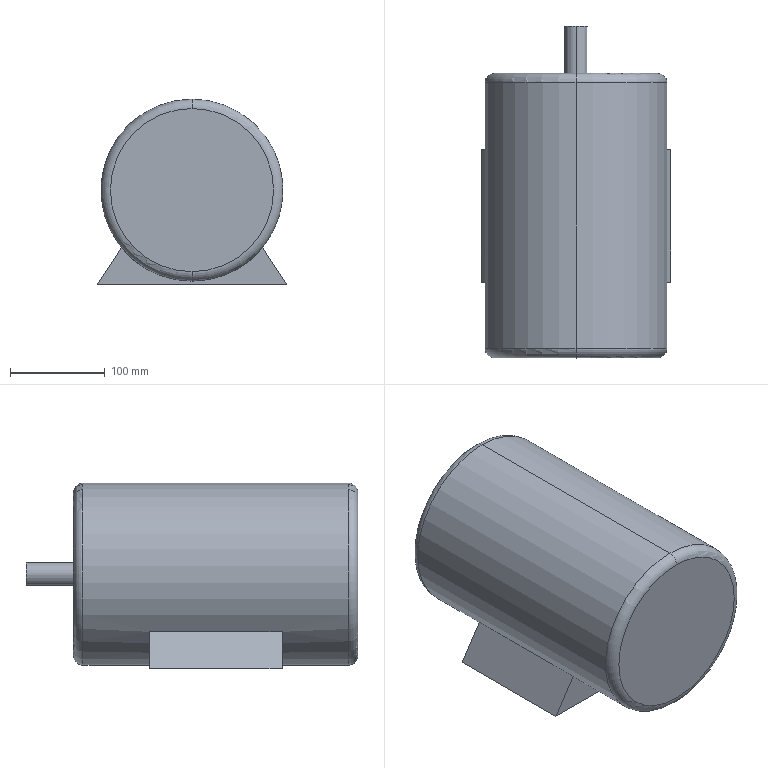Part | SolidWorks | features ICE 2, Extrusion 1, Fillet 1 | 1 solid | 16 faces | box 200 x 350 x 196 mm | volume 9129651 mm3 | plane 8 | torus 4 | cylinder 4 | commonest cylinder face diameters 24 x2 192 x2
STEP:
#1=CARTESIAN_POINT('',(0.,290.,-96.));
#2=VERTEX_POINT('',#1);
#3=CARTESIAN_POINT('',(0.,290.,96.));
#4=VERTEX_POINT('',#3);
#5=CARTESIAN_POINT('',(0.,290.,0.));
#6=DIRECTION('',(0.,-1.,0.));
#7=DIRECTION('',(0.,0.,1.));
#8=AXIS2_PLACEMENT_3D('',#5,#6,#7);
#9=CIRCLE('',#8,96.);
#10=EDGE_CURVE('',#2,#4,#9,.T.);
#11=ORIENTED_EDGE('',*,*,#10,.F.);
#12=CARTESIAN_POINT('',(0.,300.,-86.));
#13=VERTEX_POINT('',#12);
#14=CARTESIAN_POINT('',(0.,290.,-86.));
#15=DIRECTION('',(1.,0.,0.));
#16=DIRECTION('',(0.,0.,-1.));
#17=AXIS2_PLACEMENT_3D('',#14,#15,#16);
#18=CIRCLE('',#17,10.);
#19=EDGE_CURVE('',#2,#13,#18,.T.);
#20=ORIENTED_EDGE('',*,*,#19,.T.);
#21=CARTESIAN_POINT('',(0.,300.,86.));
#22=VERTEX_POINT('',#21);
#23=CARTESIAN_POINT('',(0.,300.,0.));
#24=DIRECTION('',(0.,1.,0.));
#25=DIRECTION('',(0.,0.,1.));
#26=AXIS2_PLACEMENT_3D('',#23,#24,#25);
#27=CIRCLE('',#26,86.);
#28=EDGE_CURVE('',#22,#13,#27,.T.);
#29=ORIENTED_EDGE('',*,*,#28,.F.);
#30=CARTESIAN_POINT('',(0.,290.,86.));
#31=DIRECTION('',(-1.,0.,0.));
#32=DIRECTION('',(0.,0.,1.));
#33=AXIS2_PLACEMENT_3D('',#30,#31,#32);
#34=CIRCLE('',#33,10.);
#35=EDGE_CURVE('',#4,#22,#34,.T.);
#36=ORIENTED_EDGE('',*,*,#35,.F.);
#37=EDGE_LOOP('',(#11,#20,#29,#36));
#38=FACE_OUTER_BOUND('',#37,.T.);
#39=CARTESIAN_POINT('',(0.,290.,0.));
#40=DIRECTION('',(0.,1.,0.));
#41=DIRECTION('',(0.,0.,1.));
#42=AXIS2_PLACEMENT_3D('',#39,#40,#41);
#43=TOROIDAL_SURFACE('',#42,86.,10.);
#44=ADVANCED_FACE('',(#38),#43,.T.);
#45=CARTESIAN_POINT('',(0.,0.,-86.));
#46=VERTEX_POINT('',#45);
#47=CARTESIAN_POINT('',(0.,0.,86.));
#48=VERTEX_POINT('',#47);
#49=CARTESIAN_POINT('',(0.,0.,0.));
#50=DIRECTION('',(0.,-1.,0.));
#51=DIRECTION('',(0.,0.,1.));
#52=AXIS2_PLACEMENT_3D('',#49,#50,#51);
#53=CIRCLE('',#52,86.);
#54=EDGE_CURVE('',#46,#48,#53,.T.);
#55=ORIENTED_EDGE('',*,*,#54,.F.);
#56=CARTESIAN_POINT('',(0.,10.,-96.));
#57=VERTEX_POINT('',#56);
#58=CARTESIAN_POINT('',(0.,10.,-86.));
#59=DIRECTION('',(1.,0.,0.));
#60=DIRECTION('',(0.,0.,-1.));
#61=AXIS2_PLACEMENT_3D('',#58,#59,#60);
#62=CIRCLE('',#61,10.);
#63=EDGE_CURVE('',#46,#57,#62,.T.);
#64=ORIENTED_EDGE('',*,*,#63,.T.);
#65=CARTESIAN_POINT('',(0.,10.,96.));
#66=VERTEX_POINT('',#65);
#67=CARTESIAN_POINT('',(0.,10.,0.));
#68=DIRECTION('',(0.,1.,0.));
#69=DIRECTION('',(0.,0.,1.));
#70=AXIS2_PLACEMENT_3D('',#67,#68,#69);
#71=CIRCLE('',#70,96.);
#72=EDGE_CURVE('',#66,#57,#71,.T.);
#73=ORIENTED_EDGE('',*,*,#72,.F.);
#74=CARTESIAN_POINT('',(0.,10.,86.));
#75=DIRECTION('',(-1.,0.,0.));
#76=DIRECTION('',(0.,0.,1.));
#77=AXIS2_PLACEMENT_3D('',#74,#75,#76);
#78=CIRCLE('',#77,10.);
#79=EDGE_CURVE('',#48,#66,#78,.T.);
#80=ORIENTED_EDGE('',*,*,#79,.F.);
#81=EDGE_LOOP('',(#55,#64,#73,#80));
#82=FACE_OUTER_BOUND('',#81,.T.);
#83=CARTESIAN_POINT('',(0.,10.,0.));
#84=DIRECTION('',(0.,1.,0.));
#85=DIRECTION('',(0.,0.,1.));
#86=AXIS2_PLACEMENT_3D('',#83,#84,#85);
#87=TOROIDAL_SURFACE('',#86,86.,10.);
#88=ADVANCED_FACE('',(#82),#87,.T.);
#89=CARTESIAN_POINT('',(0.,350.,12.));
#90=VERTEX_POINT('',#89);
#91=CARTESIAN_POINT('',(0.,350.,-12.));
#92=VERTEX_POINT('',#91);
#93=CARTESIAN_POINT('',(0.,350.,0.));
#94=DIRECTION('',(0.,1.,0.));
#95=DIRECTION('',(0.,0.,1.));
#96=AXIS2_PLACEMENT_3D('',#93,#94,#95);
#97=CIRCLE('',#96,12.);
#98=EDGE_CURVE('',#90,#92,#97,.T.);
#99=ORIENTED_EDGE('',*,*,#98,.F.);
#100=CARTESIAN_POINT('',(0.,300.,12.));
#101=VERTEX_POINT('',#100);
#102=CARTESIAN_POINT('',(0.,350.,12.));
#103=DIRECTION('',(0.,-1.,0.));
#104=VECTOR('',#103,1000.);
#105=LINE('',#102,#104);
#106=EDGE_CURVE('',#90,#101,#105,.T.);
#107=ORIENTED_EDGE('',*,*,#106,.T.);
#108=CARTESIAN_POINT('',(0.,300.,-12.));
#109=VERTEX_POINT('',#108);
#110=CARTESIAN_POINT('',(0.,300.,0.));
#111=DIRECTION('',(0.,1.,0.));
#112=DIRECTION('',(0.,0.,1.));
#113=AXIS2_PLACEMENT_3D('',#110,#111,#112);
#114=CIRCLE('',#113,12.);
#115=EDGE_CURVE('',#101,#109,#114,.T.);
#116=ORIENTED_EDGE('',*,*,#115,.T.);
#117=CARTESIAN_POINT('',(0.,350.,-12.));
#118=DIRECTION('',(0.,-1.,0.));
#119=VECTOR('',#118,1000.);
#120=LINE('',#117,#119);
#121=EDGE_CURVE('',#92,#109,#120,.T.);
#122=ORIENTED_EDGE('',*,*,#121,.F.);
#123=EDGE_LOOP('',(#99,#107,#116,#122));
#124=FACE_OUTER_BOUND('',#123,.T.);
#125=CARTESIAN_POINT('',(0.,350.,0.));
#126=DIRECTION('',(0.,-1.,0.));
#127=DIRECTION('',(0.,0.,-1.));
#128=AXIS2_PLACEMENT_3D('',#125,#126,#127);
#129=CYLINDRICAL_SURFACE('',#128,12.);
#130=ADVANCED_FACE('',(#124),#129,.T.);
#131=ORIENTED_EDGE('',*,*,#10,.T.);
#132=CARTESIAN_POINT('',(0.,300.,96.));
#133=DIRECTION('',(0.,-1.,0.));
#134=VECTOR('',#133,1000.);
#135=LINE('',#132,#134);
#136=EDGE_CURVE('',#4,#66,#135,.T.);
#137=ORIENTED_EDGE('',*,*,#136,.T.);
#138=ORIENTED_EDGE('',*,*,#72,.T.);
#139=CARTESIAN_POINT('',(0.,80.,-96.));
#140=VERTEX_POINT('',#139);
#141=CARTESIAN_POINT('',(0.,300.,-96.));
#142=DIRECTION('',(0.,-1.,0.));
#143=VECTOR('',#142,1000.);
#144=LINE('',#141,#143);
#145=EDGE_CURVE('',#140,#57,#144,.T.);
#146=ORIENTED_EDGE('',*,*,#145,.F.);
#147=CARTESIAN_POINT('',(74.225,80.,-60.882));
#148=VERTEX_POINT('',#147);
#149=CARTESIAN_POINT('',(0.,80.,0.));
#150=DIRECTION('',(0.,1.,0.));
#151=DIRECTION('',(0.,0.,-1.));
#152=AXIS2_PLACEMENT_3D('',#149,#150,#151);
#153=CIRCLE('',#152,96.);
#154=EDGE_CURVE('',#148,#140,#153,.T.);
#155=ORIENTED_EDGE('',*,*,#154,.F.);
#156=CARTESIAN_POINT('',(74.225,220.,-60.882));
#157=VERTEX_POINT('',#156);
#158=CARTESIAN_POINT('',(74.225,220.,-60.882));
#159=DIRECTION('',(0.,-1.,0.));
#160=VECTOR('',#159,1000.);
#161=LINE('',#158,#160);
#162=EDGE_CURVE('',#157,#148,#161,.T.);
#163=ORIENTED_EDGE('',*,*,#162,.F.);
#164=CARTESIAN_POINT('',(0.,220.,-96.));
#165=VERTEX_POINT('',#164);
#166=CARTESIAN_POINT('',(0.,220.,0.));
#167=DIRECTION('',(0.,1.,0.));
#168=DIRECTION('',(0.,0.,-1.));
#169=AXIS2_PLACEMENT_3D('',#166,#167,#168);
#170=CIRCLE('',#169,96.);
#171=EDGE_CURVE('',#157,#165,#170,.T.);
#172=ORIENTED_EDGE('',*,*,#171,.T.);
#173=CARTESIAN_POINT('',(0.,300.,-96.));
#174=DIRECTION('',(0.,-1.,0.));
#175=VECTOR('',#174,1000.);
#176=LINE('',#173,#175);
#177=EDGE_CURVE('',#2,#165,#176,.T.);
#178=ORIENTED_EDGE('',*,*,#177,.F.);
#179=EDGE_LOOP('',(#131,#137,#138,#146,#155,#163,#172,#178));
#180=FACE_OUTER_BOUND('',#179,.T.);
#181=CARTESIAN_POINT('',(0.,300.,0.));
#182=DIRECTION('',(0.,-1.,0.));
#183=DIRECTION('',(0.,0.,-1.));
#184=AXIS2_PLACEMENT_3D('',#181,#182,#183);
#185=CYLINDRICAL_SURFACE('',#184,96.);
#186=ADVANCED_FACE('',(#180),#185,.T.);
#187=ORIENTED_EDGE('',*,*,#136,.F.);
#188=CARTESIAN_POINT('',(0.,290.,0.));
#189=DIRECTION('',(0.,-1.,0.));
#190=DIRECTION('',(0.,0.,1.));
#191=AXIS2_PLACEMENT_3D('',#188,#189,#190);
#192=CIRCLE('',#191,96.);
#193=EDGE_CURVE('',#4,#2,#192,.T.);
#194=ORIENTED_EDGE('',*,*,#193,.T.);
#195=ORIENTED_EDGE('',*,*,#177,.T.);
#196=CARTESIAN_POINT('',(-74.225,220.,-60.882));
#197=VERTEX_POINT('',#196);
#198=CARTESIAN_POINT('',(0.,220.,0.));
#199=DIRECTION('',(0.,1.,0.));
#200=DIRECTION('',(0.,0.,-1.));
#201=AXIS2_PLACEMENT_3D('',#198,#199,#200);
#202=CIRCLE('',#201,96.);
#203=EDGE_CURVE('',#165,#197,#202,.T.);
#204=ORIENTED_EDGE('',*,*,#203,.T.);
#205=CARTESIAN_POINT('',(-74.225,80.,-60.882));
#206=VERTEX_POINT('',#205);
#207=CARTESIAN_POINT('',(-74.225,220.,-60.882));
#208=DIRECTION('',(0.,-1.,0.));
#209=VECTOR('',#208,1000.);
#210=LINE('',#207,#209);
#211=EDGE_CURVE('',#197,#206,#210,.T.);
#212=ORIENTED_EDGE('',*,*,#211,.T.);
#213=CARTESIAN_POINT('',(0.,80.,0.));
#214=DIRECTION('',(0.,1.,0.));
#215=DIRECTION('',(0.,0.,-1.));
#216=AXIS2_PLACEMENT_3D('',#213,#214,#215);
#217=CIRCLE('',#216,96.);
#218=EDGE_CURVE('',#140,#206,#217,.T.);
#219=ORIENTED_EDGE('',*,*,#218,.F.);
#220=ORIENTED_EDGE('',*,*,#145,.T.);
#221=CARTESIAN_POINT('',(0.,10.,0.));
#222=DIRECTION('',(0.,1.,0.));
#223=DIRECTION('',(0.,0.,1.));
#224=AXIS2_PLACEMENT_3D('',#221,#222,#223);
#225=CIRCLE('',#224,96.);
#226=EDGE_CURVE('',#57,#66,#225,.T.);
#227=ORIENTED_EDGE('',*,*,#226,.T.);
#228=EDGE_LOOP('',(#187,#194,#195,#204,#212,#219,#220,#227));
#229=FACE_OUTER_BOUND('',#228,.T.);
#230=CARTESIAN_POINT('',(0.,300.,0.));
#231=DIRECTION('',(0.,-1.,0.));
#232=DIRECTION('',(0.,0.,-1.));
#233=AXIS2_PLACEMENT_3D('',#230,#231,#232);
#234=CYLINDRICAL_SURFACE('',#233,96.);
#235=ADVANCED_FACE('',(#229),#234,.T.);
#236=ORIENTED_EDGE('',*,*,#28,.T.);
#237=CARTESIAN_POINT('',(0.,300.,0.));
#238=DIRECTION('',(0.,1.,0.));
#239=DIRECTION('',(0.,0.,1.));
#240=AXIS2_PLACEMENT_3D('',#237,#238,#239);
#241=CIRCLE('',#240,86.);
#242=EDGE_CURVE('',#13,#22,#241,.T.);
#243=ORIENTED_EDGE('',*,*,#242,.T.);
#244=EDGE_LOOP('',(#236,#243));
#245=FACE_OUTER_BOUND('',#244,.T.);
#246=CARTESIAN_POINT('',(0.,300.,0.));
#247=DIRECTION('',(0.,1.,0.));
#248=DIRECTION('',(0.,0.,1.));
#249=AXIS2_PLACEMENT_3D('',#246,#247,#248);
#250=CIRCLE('',#249,12.);
#251=EDGE_CURVE('',#109,#101,#250,.T.);
#252=ORIENTED_EDGE('',*,*,#251,.F.);
#253=ORIENTED_EDGE('',*,*,#115,.F.);
#254=EDGE_LOOP('',(#252,#253));
#255=FACE_BOUND('',#254,.T.);
#256=CARTESIAN_POINT('',(0.,300.,0.));
#257=DIRECTION('',(0.,1.,0.));
#258=DIRECTION('',(0.,0.,1.));
#259=AXIS2_PLACEMENT_3D('',#256,#257,#258);
#260=PLANE('',#259);
#261=ADVANCED_FACE('',(#245,#255),#260,.T.);
#262=CARTESIAN_POINT('',(0.,0.,0.));
#263=DIRECTION('',(0.,-1.,0.));
#264=DIRECTION('',(0.,0.,1.));
#265=AXIS2_PLACEMENT_3D('',#262,#263,#264);
#266=CIRCLE('',#265,86.);
#267=EDGE_CURVE('',#48,#46,#266,.T.);
#268=ORIENTED_EDGE('',*,*,#267,.T.);
#269=ORIENTED_EDGE('',*,*,#54,.T.);
#270=EDGE_LOOP('',(#268,#269));
#271=FACE_OUTER_BOUND('',#270,.T.);
#272=CARTESIAN_POINT('',(0.,0.,0.));
#273=DIRECTION('',(0.,1.,0.));
#274=DIRECTION('',(0.,0.,1.));
#275=AXIS2_PLACEMENT_3D('',#272,#273,#274);
#276=PLANE('',#275);
#277=ADVANCED_FACE('',(#271),#276,.F.);
#278=ORIENTED_EDGE('',*,*,#106,.F.);
#279=CARTESIAN_POINT('',(0.,350.,0.));
#280=DIRECTION('',(0.,1.,0.));
#281=DIRECTION('',(0.,0.,1.));
#282=AXIS2_PLACEMENT_3D('',#279,#280,#281);
#283=CIRCLE('',#282,12.);
#284=EDGE_CURVE('',#92,#90,#283,.T.);
#285=ORIENTED_EDGE('',*,*,#284,.F.);
#286=ORIENTED_EDGE('',*,*,#121,.T.);
#287=ORIENTED_EDGE('',*,*,#251,.T.);
#288=EDGE_LOOP('',(#278,#285,#286,#287));
#289=FACE_OUTER_BOUND('',#288,.T.);
#290=CARTESIAN_POINT('',(0.,350.,0.));
#291=DIRECTION('',(0.,-1.,0.));
#292=DIRECTION('',(0.,0.,-1.));
#293=AXIS2_PLACEMENT_3D('',#290,#291,#292);
#294=CYLINDRICAL_SURFACE('',#293,12.);
#295=ADVANCED_FACE('',(#289),#294,.T.);
#296=ORIENTED_EDGE('',*,*,#284,.T.);
#297=ORIENTED_EDGE('',*,*,#98,.T.);
#298=EDGE_LOOP('',(#296,#297));
#299=FACE_OUTER_BOUND('',#298,.T.);
#300=CARTESIAN_POINT('',(0.,350.,0.));
#301=DIRECTION('',(0.,1.,0.));
#302=DIRECTION('',(0.,0.,1.));
#303=AXIS2_PLACEMENT_3D('',#300,#301,#302);
#304=PLANE('',#303);
#305=ADVANCED_FACE('',(#299),#304,.T.);
#306=ORIENTED_EDGE('',*,*,#63,.F.);
#307=ORIENTED_EDGE('',*,*,#267,.F.);
#308=ORIENTED_EDGE('',*,*,#79,.T.);
#309=ORIENTED_EDGE('',*,*,#226,.F.);
#310=EDGE_LOOP('',(#306,#307,#308,#309));
#311=FACE_OUTER_BOUND('',#310,.T.);
#312=CARTESIAN_POINT('',(0.,10.,0.));
#313=DIRECTION('',(0.,1.,0.));
#314=DIRECTION('',(0.,0.,1.));
#315=AXIS2_PLACEMENT_3D('',#312,#313,#314);
#316=TOROIDAL_SURFACE('',#315,86.,10.);
#317=ADVANCED_FACE('',(#311),#316,.T.);
#318=ORIENTED_EDGE('',*,*,#19,.F.);
#319=ORIENTED_EDGE('',*,*,#193,.F.);
#320=ORIENTED_EDGE('',*,*,#35,.T.);
#321=ORIENTED_EDGE('',*,*,#242,.F.);
#322=EDGE_LOOP('',(#318,#319,#320,#321));
#323=FACE_OUTER_BOUND('',#322,.T.);
#324=CARTESIAN_POINT('',(0.,290.,0.));
#325=DIRECTION('',(0.,1.,0.));
#326=DIRECTION('',(0.,0.,1.));
#327=AXIS2_PLACEMENT_3D('',#324,#325,#326);
#328=TOROIDAL_SURFACE('',#327,86.,10.);
#329=ADVANCED_FACE('',(#323),#328,.T.);
#330=CARTESIAN_POINT('',(100.,80.,-100.));
#331=VERTEX_POINT('',#330);
#332=CARTESIAN_POINT('',(100.,80.,-100.));
#333=DIRECTION('',(-0.5502,0.,0.835));
#334=VECTOR('',#333,1000.);
#335=LINE('',#332,#334);
#336=EDGE_CURVE('',#331,#148,#335,.T.);
#337=ORIENTED_EDGE('',*,*,#336,.F.);
#338=CARTESIAN_POINT('',(100.,220.,-100.));
#339=VERTEX_POINT('',#338);
#340=CARTESIAN_POINT('',(100.,220.,-100.));
#341=DIRECTION('',(0.,-1.,0.));
#342=VECTOR('',#341,1000.);
#343=LINE('',#340,#342);
#344=EDGE_CURVE('',#339,#331,#343,.T.);
#345=ORIENTED_EDGE('',*,*,#344,.F.);
#346=CARTESIAN_POINT('',(100.,220.,-100.));
#347=DIRECTION('',(-0.5502,0.,0.835));
#348=VECTOR('',#347,1000.);
#349=LINE('',#346,#348);
#350=EDGE_CURVE('',#339,#157,#349,.T.);
#351=ORIENTED_EDGE('',*,*,#350,.T.);
#352=ORIENTED_EDGE('',*,*,#162,.T.);
#353=EDGE_LOOP('',(#337,#345,#351,#352));
#354=FACE_OUTER_BOUND('',#353,.T.);
#355=CARTESIAN_POINT('',(100.,220.,-100.));
#356=DIRECTION('',(0.835,0.,0.5502));
#357=DIRECTION('',(0.5502,0.,-0.835));
#358=AXIS2_PLACEMENT_3D('',#355,#356,#357);
#359=PLANE('',#358);
#360=ADVANCED_FACE('',(#354),#359,.T.);
#361=CARTESIAN_POINT('',(-100.,80.,-100.));
#362=VERTEX_POINT('',#361);
#363=CARTESIAN_POINT('',(-100.,80.,-100.));
#364=DIRECTION('',(1.,0.,0.));
#365=VECTOR('',#364,1000.);
#366=LINE('',#363,#365);
#367=EDGE_CURVE('',#362,#331,#366,.T.);
#368=ORIENTED_EDGE('',*,*,#367,.F.);
#369=CARTESIAN_POINT('',(-100.,220.,-100.));
#370=VERTEX_POINT('',#369);
#371=CARTESIAN_POINT('',(-100.,220.,-100.));
#372=DIRECTION('',(0.,-1.,0.));
#373=VECTOR('',#372,1000.);
#374=LINE('',#371,#373);
#375=EDGE_CURVE('',#370,#362,#374,.T.);
#376=ORIENTED_EDGE('',*,*,#375,.F.);
#377=CARTESIAN_POINT('',(-100.,220.,-100.));
#378=DIRECTION('',(1.,0.,0.));
#379=VECTOR('',#378,1000.);
#380=LINE('',#377,#379);
#381=EDGE_CURVE('',#370,#339,#380,.T.);
#382=ORIENTED_EDGE('',*,*,#381,.T.);
#383=ORIENTED_EDGE('',*,*,#344,.T.);
#384=EDGE_LOOP('',(#368,#376,#382,#383));
#385=FACE_OUTER_BOUND('',#384,.T.);
#386=CARTESIAN_POINT('',(-100.,220.,-100.));
#387=DIRECTION('',(0.,0.,-1.));
#388=DIRECTION('',(-1.,0.,0.));
#389=AXIS2_PLACEMENT_3D('',#386,#387,#388);
#390=PLANE('',#389);
#391=ADVANCED_FACE('',(#385),#390,.T.);
#392=CARTESIAN_POINT('',(-74.225,80.,-60.882));
#393=DIRECTION('',(-0.5502,0.,-0.835));
#394=VECTOR('',#393,1000.);
#395=LINE('',#392,#394);
#396=EDGE_CURVE('',#206,#362,#395,.T.);
#397=ORIENTED_EDGE('',*,*,#396,.F.);
#398=ORIENTED_EDGE('',*,*,#211,.F.);
#399=CARTESIAN_POINT('',(-74.225,220.,-60.882));
#400=DIRECTION('',(-0.5502,0.,-0.835));
#401=VECTOR('',#400,1000.);
#402=LINE('',#399,#401);
#403=EDGE_CURVE('',#197,#370,#402,.T.);
#404=ORIENTED_EDGE('',*,*,#403,.T.);
#405=ORIENTED_EDGE('',*,*,#375,.T.);
#406=EDGE_LOOP('',(#397,#398,#404,#405));
#407=FACE_OUTER_BOUND('',#406,.T.);
#408=CARTESIAN_POINT('',(-74.225,220.,-60.882));
#409=DIRECTION('',(-0.835,0.,0.5502));
#410=DIRECTION('',(0.5502,0.,0.835));
#411=AXIS2_PLACEMENT_3D('',#408,#409,#410);
#412=PLANE('',#411);
#413=ADVANCED_FACE('',(#407),#412,.T.);
#414=ORIENTED_EDGE('',*,*,#171,.F.);
#415=ORIENTED_EDGE('',*,*,#350,.F.);
#416=ORIENTED_EDGE('',*,*,#381,.F.);
#417=ORIENTED_EDGE('',*,*,#403,.F.);
#418=ORIENTED_EDGE('',*,*,#203,.F.);
#419=EDGE_LOOP('',(#414,#415,#416,#417,#418));
#420=FACE_OUTER_BOUND('',#419,.T.);
#421=CARTESIAN_POINT('',(0.,220.,0.));
#422=DIRECTION('',(0.,-1.,0.));
#423=DIRECTION('',(0.,0.,-1.));
#424=AXIS2_PLACEMENT_3D('',#421,#422,#423);
#425=PLANE('',#424);
#426=ADVANCED_FACE('',(#420),#425,.F.);
#427=ORIENTED_EDGE('',*,*,#154,.T.);
#428=ORIENTED_EDGE('',*,*,#218,.T.);
#429=ORIENTED_EDGE('',*,*,#396,.T.);
#430=ORIENTED_EDGE('',*,*,#367,.T.);
#431=ORIENTED_EDGE('',*,*,#336,.T.);
#432=EDGE_LOOP('',(#427,#428,#429,#430,#431));
#433=FACE_OUTER_BOUND('',#432,.T.);
#434=CARTESIAN_POINT('',(0.,80.,0.));
#435=DIRECTION('',(0.,-1.,0.));
#436=DIRECTION('',(0.,0.,-1.));
#437=AXIS2_PLACEMENT_3D('',#434,#435,#436);
#438=PLANE('',#437);
#439=ADVANCED_FACE('',(#433),#438,.T.);
#440=CLOSED_SHELL('',(#44,#88,#130,#186,#235,#261,#277,#295,#305,#317,#329,#360,#391,#413,#426,#439));
#441=MANIFOLD_SOLID_BREP('',#440);
#442=CARTESIAN_POINT('',(0.,0.,0.));
#443=DIRECTION('',(0.,0.,1.));
#444=DIRECTION('',(1.,0.,0.));
#445=AXIS2_PLACEMENT_3D('',#442,#443,#444);
#446=(LENGTH_UNIT()NAMED_UNIT(*)SI_UNIT(.MILLI.,.METRE.));
#447=UNCERTAINTY_MEASURE_WITH_UNIT(LENGTH_MEASURE(0.00001),#446,'','');
#448=(NAMED_UNIT(*)PLANE_ANGLE_UNIT()SI_UNIT($,.RADIAN.));
#449=(NAMED_UNIT(*)SI_UNIT($,.STERADIAN.)SOLID_ANGLE_UNIT());
#450=(GEOMETRIC_REPRESENTATION_CONTEXT(3)GLOBAL_UNCERTAINTY_ASSIGNED_CONTEXT((#447))GLOBAL_UNIT_ASSIGNED_CONTEXT((#446,#448,#449))REPRESENTATION_CONTEXT('',''));
#451=ADVANCED_BREP_SHAPE_REPRESENTATION('',(#441,#445),#450);